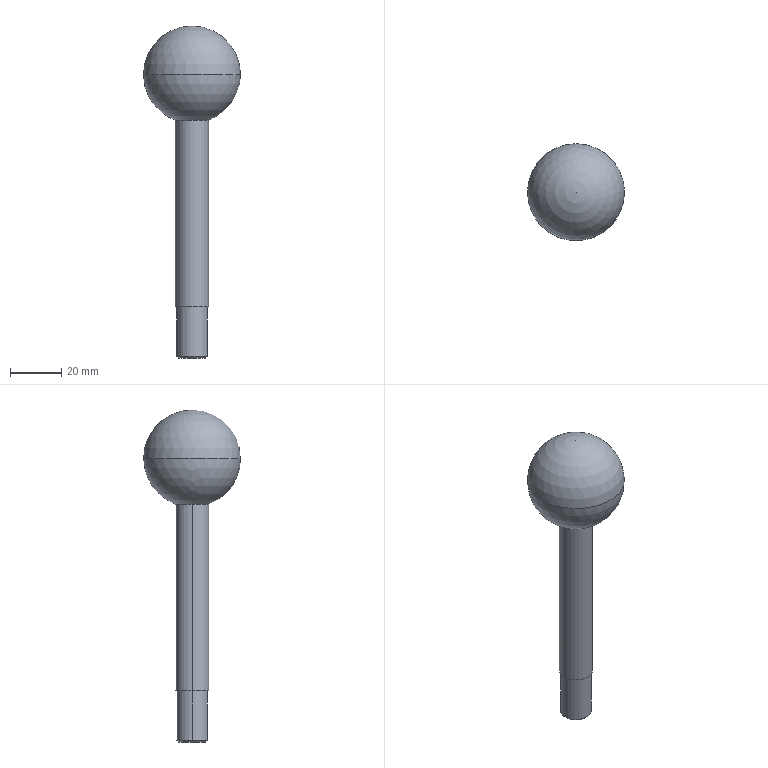Part | SolidWorks | features Revolution 2, StudWizard 1 | 1 solid | 10 faces | box 38 x 38 x 130 mm | volume 40616 mm3 | cylinder 4 | cone 2 | sphere 2 | plane 2 | commonest cylinder face diameters 12 x2 13 x2
STEP:
#1=CARTESIAN_POINT('',(5.309,0.,-111.));
#2=VERTEX_POINT('',#1);
#3=CARTESIAN_POINT('',(-5.31,0.,-111.));
#4=VERTEX_POINT('',#3);
#5=CARTESIAN_POINT('',(0.,0.,-111.));
#6=DIRECTION('',(0.,0.,1.));
#7=DIRECTION('',(1.,0.,0.));
#8=AXIS2_PLACEMENT_3D('',#5,#6,#7);
#9=CIRCLE('',#8,5.309);
#10=EDGE_CURVE('',#2,#4,#9,.T.);
#11=ORIENTED_EDGE('',*,*,#10,.T.);
#12=CARTESIAN_POINT('',(-6.,0.,-110.309));
#13=VERTEX_POINT('',#12);
#14=CARTESIAN_POINT('',(-5.309,0.,-111.));
#15=DIRECTION('',(-0.7071,0.,0.7071));
#16=VECTOR('',#15,1000.);
#17=LINE('',#14,#16);
#18=EDGE_CURVE('',#4,#13,#17,.T.);
#19=ORIENTED_EDGE('',*,*,#18,.T.);
#20=CARTESIAN_POINT('',(6.,0.,-110.309));
#21=VERTEX_POINT('',#20);
#22=CARTESIAN_POINT('',(0.,0.,-110.309));
#23=DIRECTION('',(0.,0.,1.));
#24=DIRECTION('',(1.,0.,0.));
#25=AXIS2_PLACEMENT_3D('',#22,#23,#24);
#26=CIRCLE('',#25,6.);
#27=EDGE_CURVE('',#21,#13,#26,.T.);
#28=ORIENTED_EDGE('',*,*,#27,.F.);
#29=CARTESIAN_POINT('',(5.309,0.,-111.));
#30=DIRECTION('',(0.7071,0.,0.7071));
#31=VECTOR('',#30,1000.);
#32=LINE('',#29,#31);
#33=EDGE_CURVE('',#2,#21,#32,.T.);
#34=ORIENTED_EDGE('',*,*,#33,.F.);
#35=EDGE_LOOP('',(#11,#19,#28,#34));
#36=FACE_OUTER_BOUND('',#35,.T.);
#37=CARTESIAN_POINT('',(0.,0.,-111.));
#38=DIRECTION('',(0.,0.,1.));
#39=DIRECTION('',(1.,0.,0.));
#40=AXIS2_PLACEMENT_3D('',#37,#38,#39);
#41=CONICAL_SURFACE('',#40,5.309,0.7854);
#42=ADVANCED_FACE('',(#36),#41,.T.);
#43=ORIENTED_EDGE('',*,*,#27,.T.);
#44=CARTESIAN_POINT('',(-6.,0.,-91.));
#45=VERTEX_POINT('',#44);
#46=CARTESIAN_POINT('',(-6.,0.,-111.));
#47=DIRECTION('',(0.,0.,1.));
#48=VECTOR('',#47,1000.);
#49=LINE('',#46,#48);
#50=EDGE_CURVE('',#13,#45,#49,.T.);
#51=ORIENTED_EDGE('',*,*,#50,.T.);
#52=CARTESIAN_POINT('',(6.,0.,-91.));
#53=VERTEX_POINT('',#52);
#54=CARTESIAN_POINT('',(0.,0.,-91.));
#55=DIRECTION('',(0.,0.,1.));
#56=DIRECTION('',(1.,0.,0.));
#57=AXIS2_PLACEMENT_3D('',#54,#55,#56);
#58=CIRCLE('',#57,6.);
#59=EDGE_CURVE('',#53,#45,#58,.T.);
#60=ORIENTED_EDGE('',*,*,#59,.F.);
#61=CARTESIAN_POINT('',(6.,0.,-111.));
#62=DIRECTION('',(0.,0.,1.));
#63=VECTOR('',#62,1000.);
#64=LINE('',#61,#63);
#65=EDGE_CURVE('',#21,#53,#64,.T.);
#66=ORIENTED_EDGE('',*,*,#65,.F.);
#67=EDGE_LOOP('',(#43,#51,#60,#66));
#68=FACE_OUTER_BOUND('',#67,.T.);
#69=CARTESIAN_POINT('',(0.,0.,-111.));
#70=DIRECTION('',(0.,0.,1.));
#71=DIRECTION('',(1.,0.,0.));
#72=AXIS2_PLACEMENT_3D('',#69,#70,#71);
#73=CYLINDRICAL_SURFACE('',#72,6.);
#74=ADVANCED_FACE('',(#68),#73,.T.);
#75=CARTESIAN_POINT('',(-6.5,0.,-17.854));
#76=VERTEX_POINT('',#75);
#77=CARTESIAN_POINT('',(6.5,0.,-17.854));
#78=VERTEX_POINT('',#77);
#79=CARTESIAN_POINT('',(0.,0.,-17.854));
#80=DIRECTION('',(0.,0.,-1.));
#81=DIRECTION('',(1.,0.,0.));
#82=AXIS2_PLACEMENT_3D('',#79,#80,#81);
#83=CIRCLE('',#82,6.5);
#84=EDGE_CURVE('',#76,#78,#83,.T.);
#85=ORIENTED_EDGE('',*,*,#84,.T.);
#86=CARTESIAN_POINT('',(6.5,0.,-91.));
#87=VERTEX_POINT('',#86);
#88=CARTESIAN_POINT('',(6.5,0.,-111.));
#89=DIRECTION('',(0.,0.,-1.));
#90=VECTOR('',#89,1000.);
#91=LINE('',#88,#90);
#92=EDGE_CURVE('',#78,#87,#91,.T.);
#93=ORIENTED_EDGE('',*,*,#92,.T.);
#94=CARTESIAN_POINT('',(-6.5,0.,-91.));
#95=VERTEX_POINT('',#94);
#96=CARTESIAN_POINT('',(0.,0.,-91.));
#97=DIRECTION('',(0.,0.,1.));
#98=DIRECTION('',(1.,0.,0.));
#99=AXIS2_PLACEMENT_3D('',#96,#97,#98);
#100=CIRCLE('',#99,6.5);
#101=EDGE_CURVE('',#87,#95,#100,.T.);
#102=ORIENTED_EDGE('',*,*,#101,.T.);
#103=CARTESIAN_POINT('',(-6.5,0.,-111.));
#104=DIRECTION('',(0.,0.,-1.));
#105=VECTOR('',#104,1000.);
#106=LINE('',#103,#105);
#107=EDGE_CURVE('',#76,#95,#106,.T.);
#108=ORIENTED_EDGE('',*,*,#107,.F.);
#109=EDGE_LOOP('',(#85,#93,#102,#108));
#110=FACE_OUTER_BOUND('',#109,.T.);
#111=CARTESIAN_POINT('',(0.,0.,-111.));
#112=DIRECTION('',(0.,0.,-1.));
#113=DIRECTION('',(-1.,0.,0.));
#114=AXIS2_PLACEMENT_3D('',#111,#112,#113);
#115=CYLINDRICAL_SURFACE('',#114,6.5);
#116=ADVANCED_FACE('',(#110),#115,.T.);
#117=ORIENTED_EDGE('',*,*,#84,.F.);
#118=CARTESIAN_POINT('',(0.,0.,-17.854));
#119=DIRECTION('',(0.,0.,-1.));
#120=DIRECTION('',(1.,0.,0.));
#121=AXIS2_PLACEMENT_3D('',#118,#119,#120);
#122=CIRCLE('',#121,6.5);
#123=EDGE_CURVE('',#78,#76,#122,.T.);
#124=ORIENTED_EDGE('',*,*,#123,.F.);
#125=EDGE_LOOP('',(#117,#124));
#126=FACE_BOUND('',#125,.T.);
#127=CARTESIAN_POINT('',(19.,0.,0.));
#128=VERTEX_POINT('',#127);
#129=CARTESIAN_POINT('',(-19.,0.,0.));
#130=VERTEX_POINT('',#129);
#131=CARTESIAN_POINT('',(0.,0.,0.));
#132=DIRECTION('',(0.,0.,1.));
#133=DIRECTION('',(1.,0.,0.));
#134=AXIS2_PLACEMENT_3D('',#131,#132,#133);
#135=CIRCLE('',#134,19.);
#136=EDGE_CURVE('',#128,#130,#135,.T.);
#137=ORIENTED_EDGE('',*,*,#136,.F.);
#138=CARTESIAN_POINT('',(0.,0.,0.));
#139=DIRECTION('',(0.,0.,-1.));
#140=DIRECTION('',(0.,1.,0.));
#141=AXIS2_PLACEMENT_3D('',#138,#139,#140);
#142=CIRCLE('',#141,19.);
#143=EDGE_CURVE('',#128,#130,#142,.T.);
#144=ORIENTED_EDGE('',*,*,#143,.T.);
#145=EDGE_LOOP('',(#137,#144));
#146=FACE_OUTER_BOUND('',#145,.T.);
#147=CARTESIAN_POINT('',(0.,0.,0.));
#148=DIRECTION('',(0.,0.,-1.));
#149=DIRECTION('',(0.,1.,0.));
#150=AXIS2_PLACEMENT_3D('',#147,#148,#149);
#151=SPHERICAL_SURFACE('',#150,19.);
#152=ADVANCED_FACE('',(#126,#146),#151,.T.);
#153=ORIENTED_EDGE('',*,*,#143,.F.);
#154=ORIENTED_EDGE('',*,*,#136,.T.);
#155=EDGE_LOOP('',(#153,#154));
#156=FACE_OUTER_BOUND('',#155,.T.);
#157=CARTESIAN_POINT('',(0.,0.,0.));
#158=DIRECTION('',(0.,0.,-1.));
#159=DIRECTION('',(0.,1.,0.));
#160=AXIS2_PLACEMENT_3D('',#157,#158,#159);
#161=SPHERICAL_SURFACE('',#160,19.);
#162=ADVANCED_FACE('',(#156),#161,.T.);
#163=ORIENTED_EDGE('',*,*,#92,.F.);
#164=ORIENTED_EDGE('',*,*,#123,.T.);
#165=ORIENTED_EDGE('',*,*,#107,.T.);
#166=CARTESIAN_POINT('',(0.,0.,-91.));
#167=DIRECTION('',(0.,0.,1.));
#168=DIRECTION('',(1.,0.,0.));
#169=AXIS2_PLACEMENT_3D('',#166,#167,#168);
#170=CIRCLE('',#169,6.5);
#171=EDGE_CURVE('',#95,#87,#170,.T.);
#172=ORIENTED_EDGE('',*,*,#171,.T.);
#173=EDGE_LOOP('',(#163,#164,#165,#172));
#174=FACE_OUTER_BOUND('',#173,.T.);
#175=CARTESIAN_POINT('',(0.,0.,-111.));
#176=DIRECTION('',(0.,0.,-1.));
#177=DIRECTION('',(-1.,0.,0.));
#178=AXIS2_PLACEMENT_3D('',#175,#176,#177);
#179=CYLINDRICAL_SURFACE('',#178,6.5);
#180=ADVANCED_FACE('',(#174),#179,.T.);
#181=ORIENTED_EDGE('',*,*,#50,.F.);
#182=CARTESIAN_POINT('',(0.,0.,-110.309));
#183=DIRECTION('',(0.,0.,1.));
#184=DIRECTION('',(1.,0.,0.));
#185=AXIS2_PLACEMENT_3D('',#182,#183,#184);
#186=CIRCLE('',#185,6.);
#187=EDGE_CURVE('',#13,#21,#186,.T.);
#188=ORIENTED_EDGE('',*,*,#187,.T.);
#189=ORIENTED_EDGE('',*,*,#65,.T.);
#190=CARTESIAN_POINT('',(0.,0.,-91.));
#191=DIRECTION('',(0.,0.,1.));
#192=DIRECTION('',(1.,0.,0.));
#193=AXIS2_PLACEMENT_3D('',#190,#191,#192);
#194=CIRCLE('',#193,6.);
#195=EDGE_CURVE('',#45,#53,#194,.T.);
#196=ORIENTED_EDGE('',*,*,#195,.F.);
#197=EDGE_LOOP('',(#181,#188,#189,#196));
#198=FACE_OUTER_BOUND('',#197,.T.);
#199=CARTESIAN_POINT('',(0.,0.,-111.));
#200=DIRECTION('',(0.,0.,1.));
#201=DIRECTION('',(1.,0.,0.));
#202=AXIS2_PLACEMENT_3D('',#199,#200,#201);
#203=CYLINDRICAL_SURFACE('',#202,6.);
#204=ADVANCED_FACE('',(#198),#203,.T.);
#205=ORIENTED_EDGE('',*,*,#171,.F.);
#206=ORIENTED_EDGE('',*,*,#101,.F.);
#207=EDGE_LOOP('',(#205,#206));
#208=FACE_OUTER_BOUND('',#207,.T.);
#209=ORIENTED_EDGE('',*,*,#59,.T.);
#210=ORIENTED_EDGE('',*,*,#195,.T.);
#211=EDGE_LOOP('',(#209,#210));
#212=FACE_BOUND('',#211,.T.);
#213=CARTESIAN_POINT('',(6.,0.,-91.));
#214=DIRECTION('',(0.,0.,1.));
#215=DIRECTION('',(1.,0.,0.));
#216=AXIS2_PLACEMENT_3D('',#213,#214,#215);
#217=PLANE('',#216);
#218=ADVANCED_FACE('',(#208,#212),#217,.F.);
#219=ORIENTED_EDGE('',*,*,#18,.F.);
#220=CARTESIAN_POINT('',(0.,0.,-111.));
#221=DIRECTION('',(0.,0.,1.));
#222=DIRECTION('',(1.,0.,0.));
#223=AXIS2_PLACEMENT_3D('',#220,#221,#222);
#224=CIRCLE('',#223,5.309);
#225=EDGE_CURVE('',#4,#2,#224,.T.);
#226=ORIENTED_EDGE('',*,*,#225,.T.);
#227=ORIENTED_EDGE('',*,*,#33,.T.);
#228=ORIENTED_EDGE('',*,*,#187,.F.);
#229=EDGE_LOOP('',(#219,#226,#227,#228));
#230=FACE_OUTER_BOUND('',#229,.T.);
#231=CARTESIAN_POINT('',(0.,0.,-111.));
#232=DIRECTION('',(0.,0.,1.));
#233=DIRECTION('',(1.,0.,0.));
#234=AXIS2_PLACEMENT_3D('',#231,#232,#233);
#235=CONICAL_SURFACE('',#234,5.309,0.7854);
#236=ADVANCED_FACE('',(#230),#235,.T.);
#237=ORIENTED_EDGE('',*,*,#10,.F.);
#238=ORIENTED_EDGE('',*,*,#225,.F.);
#239=EDGE_LOOP('',(#237,#238));
#240=FACE_OUTER_BOUND('',#239,.T.);
#241=CARTESIAN_POINT('',(0.,0.,-111.));
#242=DIRECTION('',(0.,0.,1.));
#243=DIRECTION('',(1.,0.,0.));
#244=AXIS2_PLACEMENT_3D('',#241,#242,#243);
#245=PLANE('',#244);
#246=ADVANCED_FACE('',(#240),#245,.F.);
#247=CLOSED_SHELL('',(#42,#74,#116,#152,#162,#180,#204,#218,#236,#246));
#248=MANIFOLD_SOLID_BREP('',#247);
#249=CARTESIAN_POINT('',(0.,0.,0.));
#250=DIRECTION('',(0.,0.,1.));
#251=DIRECTION('',(1.,0.,0.));
#252=AXIS2_PLACEMENT_3D('',#249,#250,#251);
#253=(LENGTH_UNIT()NAMED_UNIT(*)SI_UNIT(.MILLI.,.METRE.));
#254=UNCERTAINTY_MEASURE_WITH_UNIT(LENGTH_MEASURE(0.00001),#253,'','');
#255=(NAMED_UNIT(*)PLANE_ANGLE_UNIT()SI_UNIT($,.RADIAN.));
#256=(NAMED_UNIT(*)SI_UNIT($,.STERADIAN.)SOLID_ANGLE_UNIT());
#257=(GEOMETRIC_REPRESENTATION_CONTEXT(3)GLOBAL_UNCERTAINTY_ASSIGNED_CONTEXT((#254))GLOBAL_UNIT_ASSIGNED_CONTEXT((#253,#255,#256))REPRESENTATION_CONTEXT('',''));
#258=ADVANCED_BREP_SHAPE_REPRESENTATION('',(#248,#252),#257);